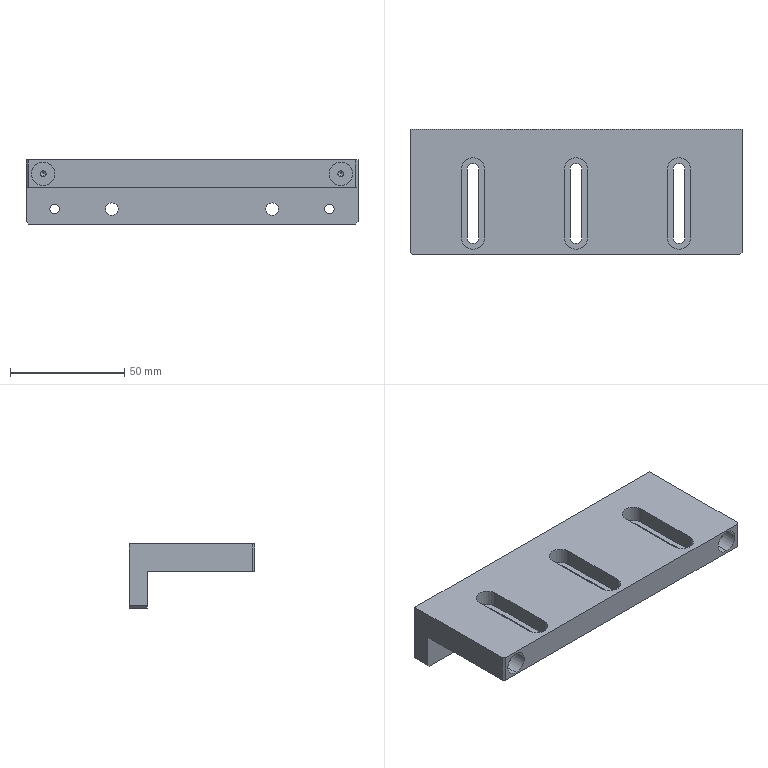Part | STEP file | 1 solid | 67 faces | box 145 x 55 x 28 mm | volume 101226 mm3 | cylinder 32 | plane 31 | cone 4 | commonest cylinder face diameters 10 x10 5.1 x6 2.5 x4 4.2 x4 5.5 x4 10.2 x4